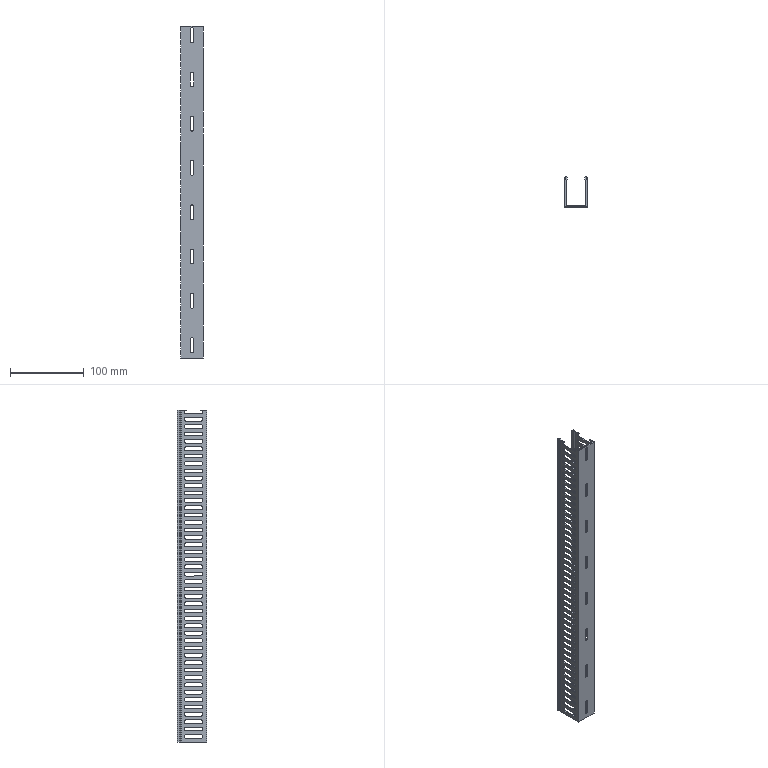Part | SolidWorks | features ICE 2, LPattern 2, Extrusion 1 | 1 solid | 523 faces | box 30 x 40 x 450 mm | volume 58936 mm3 | cylinder 307 | plane 216 | commonest cylinder face diameters 5 x294 1 x13